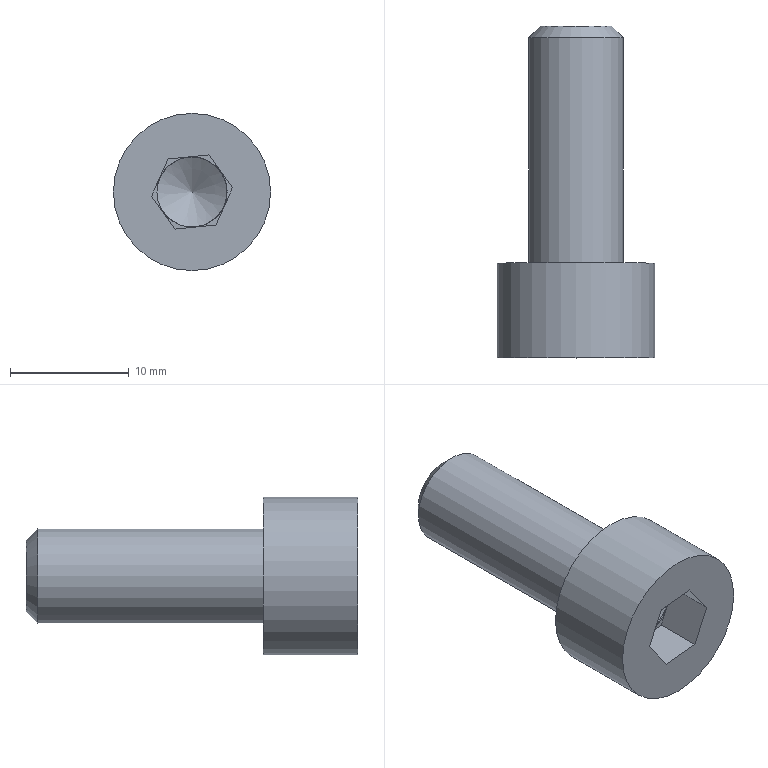Part | NX | features BOLT(M820_GB70-85) 2 | 1 solid | 15 faces | box 13.26 x 28 x 13.26 mm | volume 1958 mm3 | plane 10 | cylinder 3 | cone 2 | commonest cylinder face diameters 5.92 x1 8 x1 13.26 x1
STEP:
#1=CARTESIAN_POINT('',(833.36,-683.5,-75.));
#2=VERTEX_POINT('',#1);
#3=CARTESIAN_POINT('',(839.99,-683.5,-75.));
#4=DIRECTION('',(0.,-1.,0.));
#5=DIRECTION('',(-1.,0.,0.));
#6=AXIS2_PLACEMENT_3D('',#3,#4,#5);
#7=CIRCLE('',#6,6.63);
#8=EDGE_CURVE('',#2,#2,#7,.T.);
#9=ORIENTED_EDGE('',*,*,#8,.F.);
#10=EDGE_LOOP('',(#9));
#11=FACE_BOUND('',#10,.T.);
#12=CARTESIAN_POINT('',(835.99,-683.5,-75.));
#13=VERTEX_POINT('',#12);
#14=CARTESIAN_POINT('',(839.99,-683.5,-75.));
#15=DIRECTION('',(0.,1.,0.));
#16=DIRECTION('',(-1.,0.,0.));
#17=AXIS2_PLACEMENT_3D('',#14,#15,#16);
#18=CIRCLE('',#17,4.);
#19=EDGE_CURVE('',#13,#13,#18,.T.);
#20=ORIENTED_EDGE('',*,*,#19,.F.);
#21=EDGE_LOOP('',(#20));
#22=FACE_BOUND('',#21,.T.);
#23=CARTESIAN_POINT('',(864.667,-683.5,-105.));
#24=DIRECTION('',(0.,-1.,0.));
#25=DIRECTION('',(0.,0.,1.));
#26=AXIS2_PLACEMENT_3D('',#23,#24,#25);
#27=PLANE('',#26);
#28=ADVANCED_FACE('',(#11,#22),#27,.F.);
#29=CARTESIAN_POINT('',(837.03,-687.4,-75.));
#30=VERTEX_POINT('',#29);
#31=CARTESIAN_POINT('',(839.99,-687.4,-75.));
#32=DIRECTION('',(0.,1.,0.));
#33=DIRECTION('',(-1.,0.,0.));
#34=AXIS2_PLACEMENT_3D('',#31,#32,#33);
#35=CIRCLE('',#34,2.96);
#36=EDGE_CURVE('',#30,#30,#35,.T.);
#37=ORIENTED_EDGE('',*,*,#36,.F.);
#38=EDGE_LOOP('',(#37));
#39=FACE_BOUND('',#38,.T.);
#40=CARTESIAN_POINT('',(839.99,-685.691,-75.));
#41=VERTEX_POINT('',#40);
#42=VERTEX_LOOP('',#41);
#43=FACE_BOUND('',#42,.T.);
#44=CARTESIAN_POINT('',(839.99,-685.691,-75.));
#45=DIRECTION('',(0.,-1.,0.));
#46=DIRECTION('',(0.,0.,1.));
#47=AXIS2_PLACEMENT_3D('',#44,#45,#46);
#48=CONICAL_SURFACE('',#47,0.,1.047);
#49=ADVANCED_FACE('',(#39,#43),#48,.F.);
#50=CARTESIAN_POINT('',(837.03,-687.5,-75.));
#51=VERTEX_POINT('',#50);
#52=CARTESIAN_POINT('',(839.99,-687.5,-75.));
#53=DIRECTION('',(0.,-1.,0.));
#54=DIRECTION('',(-1.,0.,0.));
#55=AXIS2_PLACEMENT_3D('',#52,#53,#54);
#56=CIRCLE('',#55,2.96);
#57=EDGE_CURVE('',#51,#51,#56,.T.);
#58=ORIENTED_EDGE('',*,*,#57,.T.);
#59=EDGE_LOOP('',(#58));
#60=FACE_BOUND('',#59,.T.);
#61=ORIENTED_EDGE('',*,*,#36,.T.);
#62=EDGE_LOOP('',(#61));
#63=FACE_BOUND('',#62,.T.);
#64=CARTESIAN_POINT('',(839.99,-687.4,-75.));
#65=DIRECTION('',(0.,1.,0.));
#66=DIRECTION('',(0.,0.,-1.));
#67=AXIS2_PLACEMENT_3D('',#64,#65,#66);
#68=CYLINDRICAL_SURFACE('',#67,2.96);
#69=ADVANCED_FACE('',(#60,#63),#68,.F.);
#70=CARTESIAN_POINT('',(833.36,-691.5,-75.));
#71=VERTEX_POINT('',#70);
#72=CARTESIAN_POINT('',(839.99,-691.5,-75.));
#73=DIRECTION('',(0.,-1.,0.));
#74=DIRECTION('',(-1.,0.,0.));
#75=AXIS2_PLACEMENT_3D('',#72,#73,#74);
#76=CIRCLE('',#75,6.63);
#77=EDGE_CURVE('',#71,#71,#76,.T.);
#78=ORIENTED_EDGE('',*,*,#77,.F.);
#79=EDGE_LOOP('',(#78));
#80=FACE_BOUND('',#79,.T.);
#81=ORIENTED_EDGE('',*,*,#8,.T.);
#82=EDGE_LOOP('',(#81));
#83=FACE_BOUND('',#82,.T.);
#84=CARTESIAN_POINT('',(839.99,-687.5,-75.));
#85=DIRECTION('',(0.,-1.,0.));
#86=DIRECTION('',(0.,0.,1.));
#87=AXIS2_PLACEMENT_3D('',#84,#85,#86);
#88=CYLINDRICAL_SURFACE('',#87,6.63);
#89=ADVANCED_FACE('',(#80,#83),#88,.T.);
#90=ORIENTED_EDGE('',*,*,#77,.T.);
#91=EDGE_LOOP('',(#90));
#92=FACE_BOUND('',#91,.T.);
#93=CARTESIAN_POINT('',(836.577,-691.5,-75.338));
#94=VERTEX_POINT('',#93);
#95=CARTESIAN_POINT('',(838.576,-691.5,-78.125));
#96=VERTEX_POINT('',#95);
#97=CARTESIAN_POINT('',(837.577,-691.5,-76.731));
#98=DIRECTION('',(0.5829,0.,-0.8126));
#99=VECTOR('',#98,1000.);
#100=LINE('',#97,#99);
#101=EDGE_CURVE('',#94,#96,#100,.T.);
#102=ORIENTED_EDGE('',*,*,#101,.F.);
#103=CARTESIAN_POINT('',(837.991,-691.5,-72.213));
#104=VERTEX_POINT('',#103);
#105=CARTESIAN_POINT('',(837.284,-691.5,-73.775));
#106=DIRECTION('',(-0.4123,0.,-0.9111));
#107=VECTOR('',#106,1000.);
#108=LINE('',#105,#107);
#109=EDGE_CURVE('',#104,#94,#108,.T.);
#110=ORIENTED_EDGE('',*,*,#109,.F.);
#111=CARTESIAN_POINT('',(841.404,-691.5,-71.875));
#112=VERTEX_POINT('',#111);
#113=CARTESIAN_POINT('',(839.698,-691.5,-72.044));
#114=DIRECTION('',(-0.9951,0.,-0.09849));
#115=VECTOR('',#114,1000.);
#116=LINE('',#113,#115);
#117=EDGE_CURVE('',#112,#104,#116,.T.);
#118=ORIENTED_EDGE('',*,*,#117,.F.);
#119=CARTESIAN_POINT('',(843.404,-691.5,-74.662));
#120=VERTEX_POINT('',#119);
#121=CARTESIAN_POINT('',(842.404,-691.5,-73.269));
#122=DIRECTION('',(-0.5829,0.,0.8126));
#123=VECTOR('',#122,1000.);
#124=LINE('',#121,#123);
#125=EDGE_CURVE('',#120,#112,#124,.T.);
#126=ORIENTED_EDGE('',*,*,#125,.F.);
#127=CARTESIAN_POINT('',(841.99,-691.5,-77.787));
#128=VERTEX_POINT('',#127);
#129=CARTESIAN_POINT('',(842.697,-691.5,-76.225));
#130=DIRECTION('',(0.4123,0.,0.9111));
#131=VECTOR('',#130,1000.);
#132=LINE('',#129,#131);
#133=EDGE_CURVE('',#128,#120,#132,.T.);
#134=ORIENTED_EDGE('',*,*,#133,.F.);
#135=CARTESIAN_POINT('',(840.283,-691.5,-77.956));
#136=DIRECTION('',(0.9951,0.,0.09849));
#137=VECTOR('',#136,1000.);
#138=LINE('',#135,#137);
#139=EDGE_CURVE('',#96,#128,#138,.T.);
#140=ORIENTED_EDGE('',*,*,#139,.F.);
#141=EDGE_LOOP('',(#102,#110,#118,#126,#134,#140));
#142=FACE_BOUND('',#141,.T.);
#143=CARTESIAN_POINT('',(864.667,-691.5,-105.));
#144=DIRECTION('',(0.,-1.,0.));
#145=DIRECTION('',(0.,0.,1.));
#146=AXIS2_PLACEMENT_3D('',#143,#144,#145);
#147=PLANE('',#146);
#148=ADVANCED_FACE('',(#92,#142),#147,.T.);
#149=CARTESIAN_POINT('',(838.576,-687.5,-78.125));
#150=VERTEX_POINT('',#149);
#151=CARTESIAN_POINT('',(838.576,-689.5,-78.125));
#152=DIRECTION('',(0.,1.,0.));
#153=VECTOR('',#152,1000.);
#154=LINE('',#151,#153);
#155=EDGE_CURVE('',#96,#150,#154,.T.);
#156=ORIENTED_EDGE('',*,*,#155,.F.);
#157=ORIENTED_EDGE('',*,*,#139,.T.);
#158=CARTESIAN_POINT('',(841.99,-687.5,-77.787));
#159=VERTEX_POINT('',#158);
#160=CARTESIAN_POINT('',(841.99,-689.5,-77.787));
#161=DIRECTION('',(0.,1.,0.));
#162=VECTOR('',#161,1000.);
#163=LINE('',#160,#162);
#164=EDGE_CURVE('',#128,#159,#163,.T.);
#165=ORIENTED_EDGE('',*,*,#164,.T.);
#166=CARTESIAN_POINT('',(840.283,-687.5,-77.956));
#167=DIRECTION('',(0.9951,0.,0.09849));
#168=VECTOR('',#167,1000.);
#169=LINE('',#166,#168);
#170=EDGE_CURVE('',#150,#159,#169,.T.);
#171=ORIENTED_EDGE('',*,*,#170,.F.);
#172=EDGE_LOOP('',(#156,#157,#165,#171));
#173=FACE_BOUND('',#172,.T.);
#174=CARTESIAN_POINT('',(838.576,-691.5,-78.125));
#175=DIRECTION('',(-0.09849,0.,0.9951));
#176=DIRECTION('',(-0.9951,0.,-0.09849));
#177=AXIS2_PLACEMENT_3D('',#174,#175,#176);
#178=PLANE('',#177);
#179=ADVANCED_FACE('',(#173),#178,.T.);
#180=CARTESIAN_POINT('',(836.577,-687.5,-75.338));
#181=VERTEX_POINT('',#180);
#182=CARTESIAN_POINT('',(836.577,-689.5,-75.338));
#183=DIRECTION('',(0.,1.,0.));
#184=VECTOR('',#183,1000.);
#185=LINE('',#182,#184);
#186=EDGE_CURVE('',#94,#181,#185,.T.);
#187=ORIENTED_EDGE('',*,*,#186,.F.);
#188=ORIENTED_EDGE('',*,*,#101,.T.);
#189=ORIENTED_EDGE('',*,*,#155,.T.);
#190=CARTESIAN_POINT('',(837.577,-687.5,-76.731));
#191=DIRECTION('',(0.5829,0.,-0.8126));
#192=VECTOR('',#191,1000.);
#193=LINE('',#190,#192);
#194=EDGE_CURVE('',#181,#150,#193,.T.);
#195=ORIENTED_EDGE('',*,*,#194,.F.);
#196=EDGE_LOOP('',(#187,#188,#189,#195));
#197=FACE_BOUND('',#196,.T.);
#198=CARTESIAN_POINT('',(836.577,-691.5,-75.338));
#199=DIRECTION('',(0.8126,0.,0.5829));
#200=DIRECTION('',(-0.5829,0.,0.8126));
#201=AXIS2_PLACEMENT_3D('',#198,#199,#200);
#202=PLANE('',#201);
#203=ADVANCED_FACE('',(#197),#202,.T.);
#204=CARTESIAN_POINT('',(837.991,-687.5,-72.213));
#205=VERTEX_POINT('',#204);
#206=CARTESIAN_POINT('',(837.991,-689.5,-72.213));
#207=DIRECTION('',(0.,1.,0.));
#208=VECTOR('',#207,1000.);
#209=LINE('',#206,#208);
#210=EDGE_CURVE('',#104,#205,#209,.T.);
#211=ORIENTED_EDGE('',*,*,#210,.F.);
#212=ORIENTED_EDGE('',*,*,#109,.T.);
#213=ORIENTED_EDGE('',*,*,#186,.T.);
#214=CARTESIAN_POINT('',(837.284,-687.5,-73.775));
#215=DIRECTION('',(-0.4123,0.,-0.9111));
#216=VECTOR('',#215,1000.);
#217=LINE('',#214,#216);
#218=EDGE_CURVE('',#205,#181,#217,.T.);
#219=ORIENTED_EDGE('',*,*,#218,.F.);
#220=EDGE_LOOP('',(#211,#212,#213,#219));
#221=FACE_BOUND('',#220,.T.);
#222=CARTESIAN_POINT('',(837.991,-691.5,-72.213));
#223=DIRECTION('',(0.9111,0.,-0.4123));
#224=DIRECTION('',(0.4123,0.,0.9111));
#225=AXIS2_PLACEMENT_3D('',#222,#223,#224);
#226=PLANE('',#225);
#227=ADVANCED_FACE('',(#221),#226,.T.);
#228=CARTESIAN_POINT('',(841.404,-687.5,-71.875));
#229=VERTEX_POINT('',#228);
#230=CARTESIAN_POINT('',(841.404,-689.5,-71.875));
#231=DIRECTION('',(0.,1.,0.));
#232=VECTOR('',#231,1000.);
#233=LINE('',#230,#232);
#234=EDGE_CURVE('',#112,#229,#233,.T.);
#235=ORIENTED_EDGE('',*,*,#234,.F.);
#236=ORIENTED_EDGE('',*,*,#117,.T.);
#237=ORIENTED_EDGE('',*,*,#210,.T.);
#238=CARTESIAN_POINT('',(839.698,-687.5,-72.044));
#239=DIRECTION('',(-0.9951,0.,-0.09849));
#240=VECTOR('',#239,1000.);
#241=LINE('',#238,#240);
#242=EDGE_CURVE('',#229,#205,#241,.T.);
#243=ORIENTED_EDGE('',*,*,#242,.F.);
#244=EDGE_LOOP('',(#235,#236,#237,#243));
#245=FACE_BOUND('',#244,.T.);
#246=CARTESIAN_POINT('',(841.404,-691.5,-71.875));
#247=DIRECTION('',(0.09849,0.,-0.9951));
#248=DIRECTION('',(0.9951,0.,0.09849));
#249=AXIS2_PLACEMENT_3D('',#246,#247,#248);
#250=PLANE('',#249);
#251=ADVANCED_FACE('',(#245),#250,.T.);
#252=CARTESIAN_POINT('',(843.404,-687.5,-74.662));
#253=VERTEX_POINT('',#252);
#254=CARTESIAN_POINT('',(843.404,-689.5,-74.662));
#255=DIRECTION('',(0.,1.,0.));
#256=VECTOR('',#255,1000.);
#257=LINE('',#254,#256);
#258=EDGE_CURVE('',#120,#253,#257,.T.);
#259=ORIENTED_EDGE('',*,*,#258,.F.);
#260=ORIENTED_EDGE('',*,*,#125,.T.);
#261=ORIENTED_EDGE('',*,*,#234,.T.);
#262=CARTESIAN_POINT('',(842.404,-687.5,-73.269));
#263=DIRECTION('',(-0.5829,0.,0.8126));
#264=VECTOR('',#263,1000.);
#265=LINE('',#262,#264);
#266=EDGE_CURVE('',#253,#229,#265,.T.);
#267=ORIENTED_EDGE('',*,*,#266,.F.);
#268=EDGE_LOOP('',(#259,#260,#261,#267));
#269=FACE_BOUND('',#268,.T.);
#270=CARTESIAN_POINT('',(843.404,-691.5,-74.662));
#271=DIRECTION('',(-0.8126,0.,-0.5829));
#272=DIRECTION('',(0.5829,0.,-0.8126));
#273=AXIS2_PLACEMENT_3D('',#270,#271,#272);
#274=PLANE('',#273);
#275=ADVANCED_FACE('',(#269),#274,.T.);
#276=ORIENTED_EDGE('',*,*,#164,.F.);
#277=ORIENTED_EDGE('',*,*,#133,.T.);
#278=ORIENTED_EDGE('',*,*,#258,.T.);
#279=CARTESIAN_POINT('',(842.697,-687.5,-76.225));
#280=DIRECTION('',(0.4123,0.,0.9111));
#281=VECTOR('',#280,1000.);
#282=LINE('',#279,#281);
#283=EDGE_CURVE('',#159,#253,#282,.T.);
#284=ORIENTED_EDGE('',*,*,#283,.F.);
#285=EDGE_LOOP('',(#276,#277,#278,#284));
#286=FACE_BOUND('',#285,.T.);
#287=CARTESIAN_POINT('',(841.99,-691.5,-77.787));
#288=DIRECTION('',(-0.9111,0.,0.4123));
#289=DIRECTION('',(-0.4123,0.,-0.9111));
#290=AXIS2_PLACEMENT_3D('',#287,#288,#289);
#291=PLANE('',#290);
#292=ADVANCED_FACE('',(#286),#291,.T.);
#293=ORIENTED_EDGE('',*,*,#283,.T.);
#294=ORIENTED_EDGE('',*,*,#266,.T.);
#295=ORIENTED_EDGE('',*,*,#242,.T.);
#296=ORIENTED_EDGE('',*,*,#218,.T.);
#297=ORIENTED_EDGE('',*,*,#194,.T.);
#298=ORIENTED_EDGE('',*,*,#170,.T.);
#299=EDGE_LOOP('',(#293,#294,#295,#296,#297,#298));
#300=FACE_BOUND('',#299,.T.);
#301=ORIENTED_EDGE('',*,*,#57,.F.);
#302=EDGE_LOOP('',(#301));
#303=FACE_BOUND('',#302,.T.);
#304=CARTESIAN_POINT('',(864.667,-687.5,-105.));
#305=DIRECTION('',(0.,-1.,0.));
#306=DIRECTION('',(0.,0.,1.));
#307=AXIS2_PLACEMENT_3D('',#304,#305,#306);
#308=PLANE('',#307);
#309=ADVANCED_FACE('',(#300,#303),#308,.T.);
#310=CARTESIAN_POINT('',(835.99,-664.5,-75.));
#311=VERTEX_POINT('',#310);
#312=CARTESIAN_POINT('',(839.99,-664.5,-75.));
#313=DIRECTION('',(0.,1.,0.));
#314=DIRECTION('',(-1.,0.,0.));
#315=AXIS2_PLACEMENT_3D('',#312,#313,#314);
#316=CIRCLE('',#315,4.);
#317=EDGE_CURVE('',#311,#311,#316,.T.);
#318=ORIENTED_EDGE('',*,*,#317,.F.);
#319=EDGE_LOOP('',(#318));
#320=FACE_BOUND('',#319,.T.);
#321=ORIENTED_EDGE('',*,*,#19,.T.);
#322=EDGE_LOOP('',(#321));
#323=FACE_BOUND('',#322,.T.);
#324=CARTESIAN_POINT('',(839.99,-673.5,-75.));
#325=DIRECTION('',(0.,1.,0.));
#326=DIRECTION('',(0.,0.,-1.));
#327=AXIS2_PLACEMENT_3D('',#324,#325,#326);
#328=CYLINDRICAL_SURFACE('',#327,4.);
#329=ADVANCED_FACE('',(#320,#323),#328,.T.);
#330=CARTESIAN_POINT('',(836.99,-663.5,-75.));
#331=VERTEX_POINT('',#330);
#332=CARTESIAN_POINT('',(839.99,-663.5,-75.));
#333=DIRECTION('',(0.,1.,0.));
#334=DIRECTION('',(-1.,0.,0.));
#335=AXIS2_PLACEMENT_3D('',#332,#333,#334);
#336=CIRCLE('',#335,3.);
#337=EDGE_CURVE('',#331,#331,#336,.T.);
#338=ORIENTED_EDGE('',*,*,#337,.T.);
#339=EDGE_LOOP('',(#338));
#340=FACE_BOUND('',#339,.T.);
#341=CARTESIAN_POINT('',(864.667,-663.5,-105.));
#342=DIRECTION('',(0.,1.,0.));
#343=DIRECTION('',(0.,0.,-1.));
#344=AXIS2_PLACEMENT_3D('',#341,#342,#343);
#345=PLANE('',#344);
#346=ADVANCED_FACE('',(#340),#345,.T.);
#347=ORIENTED_EDGE('',*,*,#317,.T.);
#348=EDGE_LOOP('',(#347));
#349=FACE_BOUND('',#348,.T.);
#350=ORIENTED_EDGE('',*,*,#337,.F.);
#351=EDGE_LOOP('',(#350));
#352=FACE_BOUND('',#351,.T.);
#353=CARTESIAN_POINT('',(839.99,-660.5,-75.));
#354=DIRECTION('',(0.,-1.,0.));
#355=DIRECTION('',(0.,0.,1.));
#356=AXIS2_PLACEMENT_3D('',#353,#354,#355);
#357=CONICAL_SURFACE('',#356,0.,0.7854);
#358=ADVANCED_FACE('',(#349,#352),#357,.T.);
#359=CLOSED_SHELL('',(#28,#49,#69,#89,#148,#179,#203,#227,#251,#275,#292,#309,#329,#346,#358));
#360=MANIFOLD_SOLID_BREP('',#359);
#361=(LENGTH_UNIT()NAMED_UNIT(*)SI_UNIT(.MILLI.,.METRE.));
#362=UNCERTAINTY_MEASURE_WITH_UNIT(LENGTH_MEASURE(0.00001),#361,'','');
#363=(NAMED_UNIT(*)PLANE_ANGLE_UNIT()SI_UNIT($,.RADIAN.));
#364=(NAMED_UNIT(*)SI_UNIT($,.STERADIAN.)SOLID_ANGLE_UNIT());
#365=(GEOMETRIC_REPRESENTATION_CONTEXT(3)GLOBAL_UNCERTAINTY_ASSIGNED_CONTEXT((#362))GLOBAL_UNIT_ASSIGNED_CONTEXT((#361,#363,#364))REPRESENTATION_CONTEXT('',''));
#366=ADVANCED_BREP_SHAPE_REPRESENTATION('',(#360),#365);